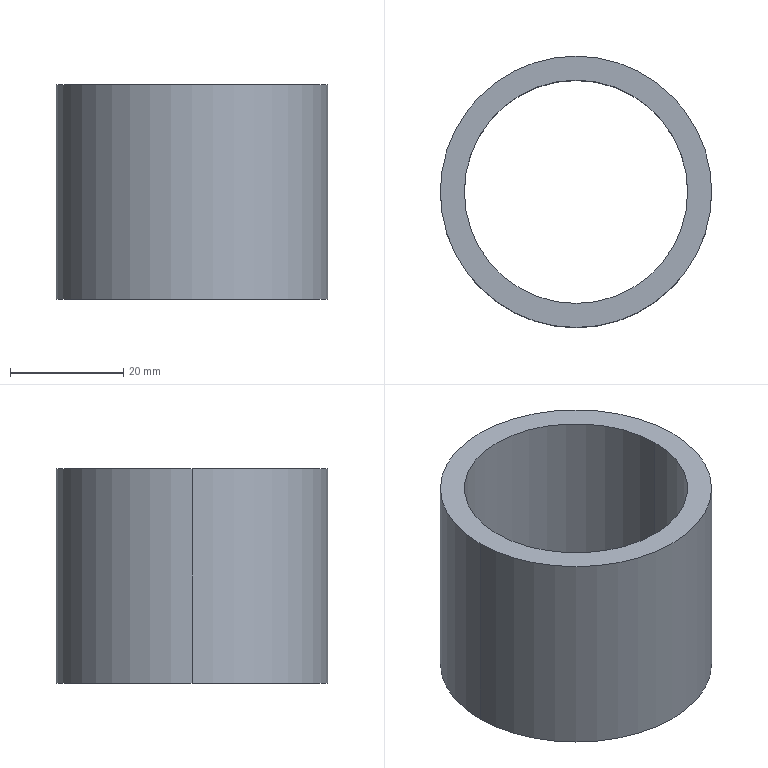Part | SolidWorks | features Extrusion 1 | 1 solid | 6 faces | box 48 x 48 x 38 mm | volume 22197 mm3 | cylinder 4 | plane 2 | commonest cylinder face diameters 39.5 x2 48 x2
STEP:
#1=CARTESIAN_POINT('',(-19.75,0.,19.));
#2=VERTEX_POINT('',#1);
#3=CARTESIAN_POINT('',(19.75,0.,19.));
#4=VERTEX_POINT('',#3);
#5=CARTESIAN_POINT('',(0.,0.,19.));
#6=DIRECTION('',(0.,0.,1.));
#7=DIRECTION('',(1.,0.,0.));
#8=AXIS2_PLACEMENT_3D('',#5,#6,#7);
#9=CIRCLE('',#8,19.75);
#10=EDGE_CURVE('',#2,#4,#9,.T.);
#11=ORIENTED_EDGE('',*,*,#10,.T.);
#12=CARTESIAN_POINT('',(19.75,0.,-19.));
#13=VERTEX_POINT('',#12);
#14=CARTESIAN_POINT('',(19.75,0.,19.));
#15=DIRECTION('',(0.,0.,-1.));
#16=VECTOR('',#15,1000.);
#17=LINE('',#14,#16);
#18=EDGE_CURVE('',#4,#13,#17,.T.);
#19=ORIENTED_EDGE('',*,*,#18,.T.);
#20=CARTESIAN_POINT('',(-19.75,0.,-19.));
#21=VERTEX_POINT('',#20);
#22=CARTESIAN_POINT('',(0.,0.,-19.));
#23=DIRECTION('',(0.,0.,1.));
#24=DIRECTION('',(1.,0.,0.));
#25=AXIS2_PLACEMENT_3D('',#22,#23,#24);
#26=CIRCLE('',#25,19.75);
#27=EDGE_CURVE('',#21,#13,#26,.T.);
#28=ORIENTED_EDGE('',*,*,#27,.F.);
#29=CARTESIAN_POINT('',(-19.75,0.,19.));
#30=DIRECTION('',(0.,0.,-1.));
#31=VECTOR('',#30,1000.);
#32=LINE('',#29,#31);
#33=EDGE_CURVE('',#2,#21,#32,.T.);
#34=ORIENTED_EDGE('',*,*,#33,.F.);
#35=EDGE_LOOP('',(#11,#19,#28,#34));
#36=FACE_OUTER_BOUND('',#35,.T.);
#37=CARTESIAN_POINT('',(0.,0.,19.));
#38=DIRECTION('',(0.,0.,-1.));
#39=DIRECTION('',(-1.,0.,0.));
#40=AXIS2_PLACEMENT_3D('',#37,#38,#39);
#41=CYLINDRICAL_SURFACE('',#40,19.75);
#42=ADVANCED_FACE('',(#36),#41,.F.);
#43=CARTESIAN_POINT('',(24.,0.,19.));
#44=VERTEX_POINT('',#43);
#45=CARTESIAN_POINT('',(-24.,0.,19.));
#46=VERTEX_POINT('',#45);
#47=CARTESIAN_POINT('',(0.,0.,19.));
#48=DIRECTION('',(0.,0.,1.));
#49=DIRECTION('',(1.,0.,0.));
#50=AXIS2_PLACEMENT_3D('',#47,#48,#49);
#51=CIRCLE('',#50,24.);
#52=EDGE_CURVE('',#44,#46,#51,.T.);
#53=ORIENTED_EDGE('',*,*,#52,.F.);
#54=CARTESIAN_POINT('',(24.,0.,-19.));
#55=VERTEX_POINT('',#54);
#56=CARTESIAN_POINT('',(24.,0.,19.));
#57=DIRECTION('',(0.,0.,-1.));
#58=VECTOR('',#57,1000.);
#59=LINE('',#56,#58);
#60=EDGE_CURVE('',#44,#55,#59,.T.);
#61=ORIENTED_EDGE('',*,*,#60,.T.);
#62=CARTESIAN_POINT('',(-24.,0.,-19.));
#63=VERTEX_POINT('',#62);
#64=CARTESIAN_POINT('',(0.,0.,-19.));
#65=DIRECTION('',(0.,0.,1.));
#66=DIRECTION('',(1.,0.,0.));
#67=AXIS2_PLACEMENT_3D('',#64,#65,#66);
#68=CIRCLE('',#67,24.);
#69=EDGE_CURVE('',#55,#63,#68,.T.);
#70=ORIENTED_EDGE('',*,*,#69,.T.);
#71=CARTESIAN_POINT('',(-24.,0.,19.));
#72=DIRECTION('',(0.,0.,-1.));
#73=VECTOR('',#72,1000.);
#74=LINE('',#71,#73);
#75=EDGE_CURVE('',#46,#63,#74,.T.);
#76=ORIENTED_EDGE('',*,*,#75,.F.);
#77=EDGE_LOOP('',(#53,#61,#70,#76));
#78=FACE_OUTER_BOUND('',#77,.T.);
#79=CARTESIAN_POINT('',(0.,0.,19.));
#80=DIRECTION('',(0.,0.,-1.));
#81=DIRECTION('',(-1.,0.,0.));
#82=AXIS2_PLACEMENT_3D('',#79,#80,#81);
#83=CYLINDRICAL_SURFACE('',#82,24.);
#84=ADVANCED_FACE('',(#78),#83,.T.);
#85=CARTESIAN_POINT('',(0.,0.,19.));
#86=DIRECTION('',(0.,0.,1.));
#87=DIRECTION('',(1.,0.,0.));
#88=AXIS2_PLACEMENT_3D('',#85,#86,#87);
#89=CIRCLE('',#88,24.);
#90=EDGE_CURVE('',#46,#44,#89,.T.);
#91=ORIENTED_EDGE('',*,*,#90,.T.);
#92=ORIENTED_EDGE('',*,*,#52,.T.);
#93=EDGE_LOOP('',(#91,#92));
#94=FACE_OUTER_BOUND('',#93,.T.);
#95=ORIENTED_EDGE('',*,*,#10,.F.);
#96=CARTESIAN_POINT('',(0.,0.,19.));
#97=DIRECTION('',(0.,0.,1.));
#98=DIRECTION('',(1.,0.,0.));
#99=AXIS2_PLACEMENT_3D('',#96,#97,#98);
#100=CIRCLE('',#99,19.75);
#101=EDGE_CURVE('',#4,#2,#100,.T.);
#102=ORIENTED_EDGE('',*,*,#101,.F.);
#103=EDGE_LOOP('',(#95,#102));
#104=FACE_BOUND('',#103,.T.);
#105=CARTESIAN_POINT('',(0.,0.,19.));
#106=DIRECTION('',(0.,0.,1.));
#107=DIRECTION('',(1.,0.,0.));
#108=AXIS2_PLACEMENT_3D('',#105,#106,#107);
#109=PLANE('',#108);
#110=ADVANCED_FACE('',(#94,#104),#109,.T.);
#111=CARTESIAN_POINT('',(0.,0.,-19.));
#112=DIRECTION('',(0.,0.,1.));
#113=DIRECTION('',(1.,0.,0.));
#114=AXIS2_PLACEMENT_3D('',#111,#112,#113);
#115=CIRCLE('',#114,24.);
#116=EDGE_CURVE('',#63,#55,#115,.T.);
#117=ORIENTED_EDGE('',*,*,#116,.F.);
#118=ORIENTED_EDGE('',*,*,#69,.F.);
#119=EDGE_LOOP('',(#117,#118));
#120=FACE_OUTER_BOUND('',#119,.T.);
#121=ORIENTED_EDGE('',*,*,#27,.T.);
#122=CARTESIAN_POINT('',(0.,0.,-19.));
#123=DIRECTION('',(0.,0.,1.));
#124=DIRECTION('',(1.,0.,0.));
#125=AXIS2_PLACEMENT_3D('',#122,#123,#124);
#126=CIRCLE('',#125,19.75);
#127=EDGE_CURVE('',#13,#21,#126,.T.);
#128=ORIENTED_EDGE('',*,*,#127,.T.);
#129=EDGE_LOOP('',(#121,#128));
#130=FACE_BOUND('',#129,.T.);
#131=CARTESIAN_POINT('',(0.,0.,-19.));
#132=DIRECTION('',(0.,0.,1.));
#133=DIRECTION('',(1.,0.,0.));
#134=AXIS2_PLACEMENT_3D('',#131,#132,#133);
#135=PLANE('',#134);
#136=ADVANCED_FACE('',(#120,#130),#135,.F.);
#137=ORIENTED_EDGE('',*,*,#60,.F.);
#138=ORIENTED_EDGE('',*,*,#90,.F.);
#139=ORIENTED_EDGE('',*,*,#75,.T.);
#140=ORIENTED_EDGE('',*,*,#116,.T.);
#141=EDGE_LOOP('',(#137,#138,#139,#140));
#142=FACE_OUTER_BOUND('',#141,.T.);
#143=CARTESIAN_POINT('',(0.,0.,19.));
#144=DIRECTION('',(0.,0.,-1.));
#145=DIRECTION('',(-1.,0.,0.));
#146=AXIS2_PLACEMENT_3D('',#143,#144,#145);
#147=CYLINDRICAL_SURFACE('',#146,24.);
#148=ADVANCED_FACE('',(#142),#147,.T.);
#149=ORIENTED_EDGE('',*,*,#18,.F.);
#150=ORIENTED_EDGE('',*,*,#101,.T.);
#151=ORIENTED_EDGE('',*,*,#33,.T.);
#152=ORIENTED_EDGE('',*,*,#127,.F.);
#153=EDGE_LOOP('',(#149,#150,#151,#152));
#154=FACE_OUTER_BOUND('',#153,.T.);
#155=CARTESIAN_POINT('',(0.,0.,19.));
#156=DIRECTION('',(0.,0.,-1.));
#157=DIRECTION('',(-1.,0.,0.));
#158=AXIS2_PLACEMENT_3D('',#155,#156,#157);
#159=CYLINDRICAL_SURFACE('',#158,19.75);
#160=ADVANCED_FACE('',(#154),#159,.F.);
#161=CLOSED_SHELL('',(#42,#84,#110,#136,#148,#160));
#162=MANIFOLD_SOLID_BREP('',#161);
#163=CARTESIAN_POINT('',(0.,0.,0.));
#164=DIRECTION('',(0.,0.,1.));
#165=DIRECTION('',(1.,0.,0.));
#166=AXIS2_PLACEMENT_3D('',#163,#164,#165);
#167=(LENGTH_UNIT()NAMED_UNIT(*)SI_UNIT(.MILLI.,.METRE.));
#168=UNCERTAINTY_MEASURE_WITH_UNIT(LENGTH_MEASURE(0.00001),#167,'','');
#169=(NAMED_UNIT(*)PLANE_ANGLE_UNIT()SI_UNIT($,.RADIAN.));
#170=(NAMED_UNIT(*)SI_UNIT($,.STERADIAN.)SOLID_ANGLE_UNIT());
#171=(GEOMETRIC_REPRESENTATION_CONTEXT(3)GLOBAL_UNCERTAINTY_ASSIGNED_CONTEXT((#168))GLOBAL_UNIT_ASSIGNED_CONTEXT((#167,#169,#170))REPRESENTATION_CONTEXT('',''));
#172=ADVANCED_BREP_SHAPE_REPRESENTATION('',(#162,#166),#171);